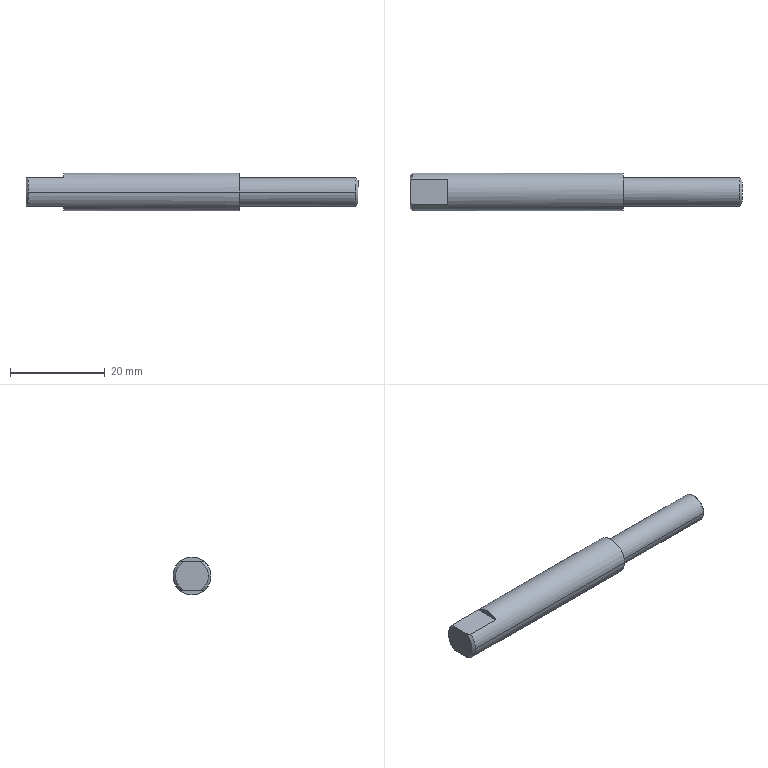Part | STEP file | 11-FG-B02611 | 1 solid | 15 faces | box 70 x 8 x 8 mm | volume 2907 mm3 | plane 7 | cylinder 4 | cone 4 | commonest cylinder face diameters 6 x2 8 x2
STEP:
#1=CARTESIAN_POINT('',(194.107,167.808,0.));
#2=VERTEX_POINT('',#1);
#3=CARTESIAN_POINT('',(194.107,175.808,0.));
#4=VERTEX_POINT('',#3);
#5=CARTESIAN_POINT('',(194.107,171.808,0.));
#6=DIRECTION('',(1.,0.,0.));
#7=DIRECTION('',(0.,0.,1.));
#8=AXIS2_PLACEMENT_3D('',#5,#6,#7);
#9=CIRCLE('',#8,4.);
#10=EDGE_CURVE('',#2,#4,#9,.T.);
#11=ORIENTED_EDGE('',*,*,#10,.F.);
#12=CARTESIAN_POINT('',(149.607,167.808,0.));
#13=VERTEX_POINT('',#12);
#14=CARTESIAN_POINT('',(194.107,167.808,0.));
#15=DIRECTION('',(-1.,0.,0.));
#16=VECTOR('',#15,1000.);
#17=LINE('',#14,#16);
#18=EDGE_CURVE('',#2,#13,#17,.T.);
#19=ORIENTED_EDGE('',*,*,#18,.T.);
#20=CARTESIAN_POINT('',(149.607,169.162,-3.));
#21=VERTEX_POINT('',#20);
#22=CARTESIAN_POINT('',(149.607,171.808,0.));
#23=DIRECTION('',(1.,0.,0.));
#24=DIRECTION('',(0.,0.,1.));
#25=AXIS2_PLACEMENT_3D('',#22,#23,#24);
#26=CIRCLE('',#25,4.);
#27=EDGE_CURVE('',#13,#21,#26,.T.);
#28=ORIENTED_EDGE('',*,*,#27,.T.);
#29=CARTESIAN_POINT('',(157.107,169.162,-3.));
#30=VERTEX_POINT('',#29);
#31=CARTESIAN_POINT('',(194.107,169.162,-3.));
#32=DIRECTION('',(1.,0.,0.));
#33=VECTOR('',#32,1000.);
#34=LINE('',#31,#33);
#35=EDGE_CURVE('',#21,#30,#34,.T.);
#36=ORIENTED_EDGE('',*,*,#35,.T.);
#37=CARTESIAN_POINT('',(157.107,174.454,-3.));
#38=VERTEX_POINT('',#37);
#39=CARTESIAN_POINT('',(157.107,171.808,0.));
#40=DIRECTION('',(1.,0.,0.));
#41=DIRECTION('',(0.,0.,1.));
#42=AXIS2_PLACEMENT_3D('',#39,#40,#41);
#43=CIRCLE('',#42,4.);
#44=EDGE_CURVE('',#30,#38,#43,.T.);
#45=ORIENTED_EDGE('',*,*,#44,.T.);
#46=CARTESIAN_POINT('',(149.607,174.454,-3.));
#47=VERTEX_POINT('',#46);
#48=CARTESIAN_POINT('',(194.107,174.454,-3.));
#49=DIRECTION('',(-1.,0.,0.));
#50=VECTOR('',#49,1000.);
#51=LINE('',#48,#50);
#52=EDGE_CURVE('',#38,#47,#51,.T.);
#53=ORIENTED_EDGE('',*,*,#52,.T.);
#54=CARTESIAN_POINT('',(149.607,175.808,0.));
#55=VERTEX_POINT('',#54);
#56=CARTESIAN_POINT('',(149.607,171.808,0.));
#57=DIRECTION('',(1.,0.,0.));
#58=DIRECTION('',(0.,0.,1.));
#59=AXIS2_PLACEMENT_3D('',#56,#57,#58);
#60=CIRCLE('',#59,4.);
#61=EDGE_CURVE('',#47,#55,#60,.T.);
#62=ORIENTED_EDGE('',*,*,#61,.T.);
#63=CARTESIAN_POINT('',(194.107,175.808,0.));
#64=DIRECTION('',(-1.,0.,0.));
#65=VECTOR('',#64,1000.);
#66=LINE('',#63,#65);
#67=EDGE_CURVE('',#4,#55,#66,.T.);
#68=ORIENTED_EDGE('',*,*,#67,.F.);
#69=EDGE_LOOP('',(#11,#19,#28,#36,#45,#53,#62,#68));
#70=FACE_OUTER_BOUND('',#69,.T.);
#71=CARTESIAN_POINT('',(194.107,171.808,0.));
#72=DIRECTION('',(-1.,0.,0.));
#73=DIRECTION('',(0.,1.,0.));
#74=AXIS2_PLACEMENT_3D('',#71,#72,#73);
#75=CYLINDRICAL_SURFACE('',#74,4.);
#76=ADVANCED_FACE('',(#70),#75,.T.);
#77=CARTESIAN_POINT('',(218.607,168.808,0.));
#78=VERTEX_POINT('',#77);
#79=CARTESIAN_POINT('',(218.607,171.808,-3.));
#80=VERTEX_POINT('',#79);
#81=CARTESIAN_POINT('',(218.607,171.808,0.));
#82=DIRECTION('',(1.,0.,0.));
#83=DIRECTION('',(0.,0.,1.));
#84=AXIS2_PLACEMENT_3D('',#81,#82,#83);
#85=CIRCLE('',#84,3.);
#86=EDGE_CURVE('',#78,#80,#85,.T.);
#87=ORIENTED_EDGE('',*,*,#86,.F.);
#88=CARTESIAN_POINT('',(194.107,168.808,0.));
#89=VERTEX_POINT('',#88);
#90=CARTESIAN_POINT('',(218.607,168.808,0.));
#91=DIRECTION('',(-1.,0.,0.));
#92=VECTOR('',#91,1000.);
#93=LINE('',#90,#92);
#94=EDGE_CURVE('',#78,#89,#93,.T.);
#95=ORIENTED_EDGE('',*,*,#94,.T.);
#96=CARTESIAN_POINT('',(194.107,174.808,0.));
#97=VERTEX_POINT('',#96);
#98=CARTESIAN_POINT('',(194.107,171.808,0.));
#99=DIRECTION('',(1.,0.,0.));
#100=DIRECTION('',(0.,0.,1.));
#101=AXIS2_PLACEMENT_3D('',#98,#99,#100);
#102=CIRCLE('',#101,3.);
#103=EDGE_CURVE('',#89,#97,#102,.T.);
#104=ORIENTED_EDGE('',*,*,#103,.T.);
#105=CARTESIAN_POINT('',(218.607,174.808,0.));
#106=VERTEX_POINT('',#105);
#107=CARTESIAN_POINT('',(218.607,174.808,0.));
#108=DIRECTION('',(-1.,0.,0.));
#109=VECTOR('',#108,1000.);
#110=LINE('',#107,#109);
#111=EDGE_CURVE('',#106,#97,#110,.T.);
#112=ORIENTED_EDGE('',*,*,#111,.F.);
#113=CARTESIAN_POINT('',(218.607,171.808,0.));
#114=DIRECTION('',(1.,0.,0.));
#115=DIRECTION('',(0.,0.,1.));
#116=AXIS2_PLACEMENT_3D('',#113,#114,#115);
#117=CIRCLE('',#116,3.);
#118=EDGE_CURVE('',#80,#106,#117,.T.);
#119=ORIENTED_EDGE('',*,*,#118,.F.);
#120=EDGE_LOOP('',(#87,#95,#104,#112,#119));
#121=FACE_OUTER_BOUND('',#120,.T.);
#122=CARTESIAN_POINT('',(218.607,171.808,0.));
#123=DIRECTION('',(-1.,0.,0.));
#124=DIRECTION('',(0.,1.,0.));
#125=AXIS2_PLACEMENT_3D('',#122,#123,#124);
#126=CYLINDRICAL_SURFACE('',#125,3.);
#127=ADVANCED_FACE('',(#121),#126,.T.);
#128=CARTESIAN_POINT('',(219.107,171.808,-2.5));
#129=VERTEX_POINT('',#128);
#130=CARTESIAN_POINT('',(219.107,171.808,2.5));
#131=VERTEX_POINT('',#130);
#132=CARTESIAN_POINT('',(219.107,171.808,0.));
#133=DIRECTION('',(1.,0.,0.));
#134=DIRECTION('',(0.,0.,1.));
#135=AXIS2_PLACEMENT_3D('',#132,#133,#134);
#136=CIRCLE('',#135,2.5);
#137=EDGE_CURVE('',#129,#131,#136,.T.);
#138=ORIENTED_EDGE('',*,*,#137,.F.);
#139=CARTESIAN_POINT('',(219.107,171.808,-2.5));
#140=DIRECTION('',(-0.7071,0.,-0.7071));
#141=VECTOR('',#140,1000.);
#142=LINE('',#139,#141);
#143=EDGE_CURVE('',#129,#80,#142,.T.);
#144=ORIENTED_EDGE('',*,*,#143,.T.);
#145=ORIENTED_EDGE('',*,*,#118,.T.);
#146=CARTESIAN_POINT('',(218.607,171.808,3.));
#147=VERTEX_POINT('',#146);
#148=CARTESIAN_POINT('',(218.607,171.808,0.));
#149=DIRECTION('',(1.,0.,0.));
#150=DIRECTION('',(0.,0.,1.));
#151=AXIS2_PLACEMENT_3D('',#148,#149,#150);
#152=CIRCLE('',#151,3.);
#153=EDGE_CURVE('',#106,#147,#152,.T.);
#154=ORIENTED_EDGE('',*,*,#153,.T.);
#155=CARTESIAN_POINT('',(219.107,171.808,2.5));
#156=DIRECTION('',(-0.7071,0.,0.7071));
#157=VECTOR('',#156,1000.);
#158=LINE('',#155,#157);
#159=EDGE_CURVE('',#131,#147,#158,.T.);
#160=ORIENTED_EDGE('',*,*,#159,.F.);
#161=EDGE_LOOP('',(#138,#144,#145,#154,#160));
#162=FACE_OUTER_BOUND('',#161,.T.);
#163=CARTESIAN_POINT('',(219.107,171.808,0.));
#164=DIRECTION('',(-1.,0.,0.));
#165=DIRECTION('',(0.,0.,1.));
#166=AXIS2_PLACEMENT_3D('',#163,#164,#165);
#167=CONICAL_SURFACE('',#166,2.5,0.7854);
#168=ADVANCED_FACE('',(#162),#167,.T.);
#169=CARTESIAN_POINT('',(219.107,171.808,0.));
#170=DIRECTION('',(1.,0.,0.));
#171=DIRECTION('',(0.,0.,1.));
#172=AXIS2_PLACEMENT_3D('',#169,#170,#171);
#173=CIRCLE('',#172,2.5);
#174=EDGE_CURVE('',#131,#129,#173,.T.);
#175=ORIENTED_EDGE('',*,*,#174,.T.);
#176=ORIENTED_EDGE('',*,*,#137,.T.);
#177=EDGE_LOOP('',(#175,#176));
#178=FACE_OUTER_BOUND('',#177,.T.);
#179=CARTESIAN_POINT('',(219.107,174.308,2.5));
#180=DIRECTION('',(1.,0.,0.));
#181=DIRECTION('',(0.,-1.,0.));
#182=AXIS2_PLACEMENT_3D('',#179,#180,#181);
#183=PLANE('',#182);
#184=ADVANCED_FACE('',(#178),#183,.T.);
#185=ORIENTED_EDGE('',*,*,#143,.F.);
#186=ORIENTED_EDGE('',*,*,#174,.F.);
#187=ORIENTED_EDGE('',*,*,#159,.T.);
#188=CARTESIAN_POINT('',(218.607,171.808,0.));
#189=DIRECTION('',(1.,0.,0.));
#190=DIRECTION('',(0.,0.,1.));
#191=AXIS2_PLACEMENT_3D('',#188,#189,#190);
#192=CIRCLE('',#191,3.);
#193=EDGE_CURVE('',#147,#78,#192,.T.);
#194=ORIENTED_EDGE('',*,*,#193,.T.);
#195=ORIENTED_EDGE('',*,*,#86,.T.);
#196=EDGE_LOOP('',(#185,#186,#187,#194,#195));
#197=FACE_OUTER_BOUND('',#196,.T.);
#198=CARTESIAN_POINT('',(219.107,171.808,0.));
#199=DIRECTION('',(-1.,0.,0.));
#200=DIRECTION('',(0.,0.,1.));
#201=AXIS2_PLACEMENT_3D('',#198,#199,#200);
#202=CONICAL_SURFACE('',#201,2.5,0.7854);
#203=ADVANCED_FACE('',(#197),#202,.T.);
#204=ORIENTED_EDGE('',*,*,#94,.F.);
#205=ORIENTED_EDGE('',*,*,#193,.F.);
#206=ORIENTED_EDGE('',*,*,#153,.F.);
#207=ORIENTED_EDGE('',*,*,#111,.T.);
#208=CARTESIAN_POINT('',(194.107,171.808,0.));
#209=DIRECTION('',(1.,0.,0.));
#210=DIRECTION('',(0.,0.,1.));
#211=AXIS2_PLACEMENT_3D('',#208,#209,#210);
#212=CIRCLE('',#211,3.);
#213=EDGE_CURVE('',#97,#89,#212,.T.);
#214=ORIENTED_EDGE('',*,*,#213,.T.);
#215=EDGE_LOOP('',(#204,#205,#206,#207,#214));
#216=FACE_OUTER_BOUND('',#215,.T.);
#217=CARTESIAN_POINT('',(218.607,171.808,0.));
#218=DIRECTION('',(-1.,0.,0.));
#219=DIRECTION('',(0.,1.,0.));
#220=AXIS2_PLACEMENT_3D('',#217,#218,#219);
#221=CYLINDRICAL_SURFACE('',#220,3.);
#222=ADVANCED_FACE('',(#216),#221,.T.);
#223=ORIENTED_EDGE('',*,*,#213,.F.);
#224=ORIENTED_EDGE('',*,*,#103,.F.);
#225=EDGE_LOOP('',(#223,#224));
#226=FACE_BOUND('',#225,.T.);
#227=CARTESIAN_POINT('',(194.107,171.808,0.));
#228=DIRECTION('',(1.,0.,0.));
#229=DIRECTION('',(0.,0.,1.));
#230=AXIS2_PLACEMENT_3D('',#227,#228,#229);
#231=CIRCLE('',#230,4.);
#232=EDGE_CURVE('',#4,#2,#231,.T.);
#233=ORIENTED_EDGE('',*,*,#232,.T.);
#234=ORIENTED_EDGE('',*,*,#10,.T.);
#235=EDGE_LOOP('',(#233,#234));
#236=FACE_OUTER_BOUND('',#235,.T.);
#237=CARTESIAN_POINT('',(194.107,175.808,4.));
#238=DIRECTION('',(1.,0.,0.));
#239=DIRECTION('',(0.,-1.,0.));
#240=AXIS2_PLACEMENT_3D('',#237,#238,#239);
#241=PLANE('',#240);
#242=ADVANCED_FACE('',(#226,#236),#241,.T.);
#243=ORIENTED_EDGE('',*,*,#18,.F.);
#244=ORIENTED_EDGE('',*,*,#232,.F.);
#245=ORIENTED_EDGE('',*,*,#67,.T.);
#246=CARTESIAN_POINT('',(149.607,174.454,3.));
#247=VERTEX_POINT('',#246);
#248=CARTESIAN_POINT('',(149.607,171.808,0.));
#249=DIRECTION('',(1.,0.,0.));
#250=DIRECTION('',(0.,0.,1.));
#251=AXIS2_PLACEMENT_3D('',#248,#249,#250);
#252=CIRCLE('',#251,4.);
#253=EDGE_CURVE('',#55,#247,#252,.T.);
#254=ORIENTED_EDGE('',*,*,#253,.T.);
#255=CARTESIAN_POINT('',(157.107,174.454,3.));
#256=VERTEX_POINT('',#255);
#257=CARTESIAN_POINT('',(194.107,174.454,3.));
#258=DIRECTION('',(1.,0.,0.));
#259=VECTOR('',#258,1000.);
#260=LINE('',#257,#259);
#261=EDGE_CURVE('',#247,#256,#260,.T.);
#262=ORIENTED_EDGE('',*,*,#261,.T.);
#263=CARTESIAN_POINT('',(157.107,169.162,3.));
#264=VERTEX_POINT('',#263);
#265=CARTESIAN_POINT('',(157.107,171.808,0.));
#266=DIRECTION('',(1.,0.,0.));
#267=DIRECTION('',(0.,0.,1.));
#268=AXIS2_PLACEMENT_3D('',#265,#266,#267);
#269=CIRCLE('',#268,4.);
#270=EDGE_CURVE('',#256,#264,#269,.T.);
#271=ORIENTED_EDGE('',*,*,#270,.T.);
#272=CARTESIAN_POINT('',(149.607,169.162,3.));
#273=VERTEX_POINT('',#272);
#274=CARTESIAN_POINT('',(194.107,169.162,3.));
#275=DIRECTION('',(-1.,0.,0.));
#276=VECTOR('',#275,1000.);
#277=LINE('',#274,#276);
#278=EDGE_CURVE('',#264,#273,#277,.T.);
#279=ORIENTED_EDGE('',*,*,#278,.T.);
#280=CARTESIAN_POINT('',(149.607,171.808,0.));
#281=DIRECTION('',(1.,0.,0.));
#282=DIRECTION('',(0.,0.,1.));
#283=AXIS2_PLACEMENT_3D('',#280,#281,#282);
#284=CIRCLE('',#283,4.);
#285=EDGE_CURVE('',#273,#13,#284,.T.);
#286=ORIENTED_EDGE('',*,*,#285,.T.);
#287=EDGE_LOOP('',(#243,#244,#245,#254,#262,#271,#279,#286));
#288=FACE_OUTER_BOUND('',#287,.T.);
#289=CARTESIAN_POINT('',(194.107,171.808,0.));
#290=DIRECTION('',(-1.,0.,0.));
#291=DIRECTION('',(0.,1.,0.));
#292=AXIS2_PLACEMENT_3D('',#289,#290,#291);
#293=CYLINDRICAL_SURFACE('',#292,4.);
#294=ADVANCED_FACE('',(#288),#293,.T.);
#295=CARTESIAN_POINT('',(149.107,170.005,-3.));
#296=VERTEX_POINT('',#295);
#297=CARTESIAN_POINT('',(149.107,170.005,-3.));
#298=CARTESIAN_POINT('',(149.257,169.714,-3.));
#299=CARTESIAN_POINT('',(149.426,169.435,-3.));
#300=CARTESIAN_POINT('',(149.607,169.162,-3.));
#301=B_SPLINE_CURVE_WITH_KNOTS('',3,(#297,#298,#299,#300),.UNSPECIFIED.,.F.,.F.,(4,4),(0.,0.0009801),.UNSPECIFIED.);
#302=EDGE_CURVE('',#296,#21,#301,.T.);
#303=ORIENTED_EDGE('',*,*,#302,.F.);
#304=CARTESIAN_POINT('',(149.107,173.611,-3.));
#305=VERTEX_POINT('',#304);
#306=CARTESIAN_POINT('',(149.107,167.805,-3.));
#307=DIRECTION('',(0.,-1.,0.));
#308=VECTOR('',#307,1000.);
#309=LINE('',#306,#308);
#310=EDGE_CURVE('',#305,#296,#309,.T.);
#311=ORIENTED_EDGE('',*,*,#310,.F.);
#312=CARTESIAN_POINT('',(149.607,174.454,-3.));
#313=CARTESIAN_POINT('',(149.426,174.181,-3.));
#314=CARTESIAN_POINT('',(149.257,173.902,-3.));
#315=CARTESIAN_POINT('',(149.107,173.611,-3.));
#316=B_SPLINE_CURVE_WITH_KNOTS('',3,(#312,#313,#314,#315),.UNSPECIFIED.,.F.,.F.,(4,4),(0.,0.0009801),.UNSPECIFIED.);
#317=EDGE_CURVE('',#47,#305,#316,.T.);
#318=ORIENTED_EDGE('',*,*,#317,.F.);
#319=ORIENTED_EDGE('',*,*,#52,.F.);
#320=CARTESIAN_POINT('',(157.107,174.954,-3.));
#321=DIRECTION('',(0.,1.,0.));
#322=VECTOR('',#321,1000.);
#323=LINE('',#320,#322);
#324=EDGE_CURVE('',#30,#38,#323,.T.);
#325=ORIENTED_EDGE('',*,*,#324,.F.);
#326=ORIENTED_EDGE('',*,*,#35,.F.);
#327=EDGE_LOOP('',(#303,#311,#318,#319,#325,#326));
#328=FACE_OUTER_BOUND('',#327,.T.);
#329=CARTESIAN_POINT('',(149.101,174.458,-3.));
#330=DIRECTION('',(0.,0.,1.));
#331=DIRECTION('',(0.,-1.,0.));
#332=AXIS2_PLACEMENT_3D('',#329,#330,#331);
#333=PLANE('',#332);
#334=ADVANCED_FACE('',(#328),#333,.F.);
#335=ORIENTED_EDGE('',*,*,#44,.F.);
#336=ORIENTED_EDGE('',*,*,#324,.T.);
#337=EDGE_LOOP('',(#335,#336));
#338=FACE_OUTER_BOUND('',#337,.T.);
#339=CARTESIAN_POINT('',(157.107,174.954,-4.502));
#340=DIRECTION('',(-1.,0.,0.));
#341=DIRECTION('',(0.,-1.,0.));
#342=AXIS2_PLACEMENT_3D('',#339,#340,#341);
#343=PLANE('',#342);
#344=ADVANCED_FACE('',(#338),#343,.T.);
#345=CARTESIAN_POINT('',(149.107,170.005,3.));
#346=VERTEX_POINT('',#345);
#347=CARTESIAN_POINT('',(149.607,169.162,3.));
#348=CARTESIAN_POINT('',(149.426,169.435,3.));
#349=CARTESIAN_POINT('',(149.257,169.714,3.));
#350=CARTESIAN_POINT('',(149.107,170.005,3.));
#351=B_SPLINE_CURVE_WITH_KNOTS('',3,(#347,#348,#349,#350),.UNSPECIFIED.,.F.,.F.,(4,4),(0.,0.0009801),.UNSPECIFIED.);
#352=EDGE_CURVE('',#273,#346,#351,.T.);
#353=ORIENTED_EDGE('',*,*,#352,.T.);
#354=CARTESIAN_POINT('',(149.107,171.808,0.));
#355=DIRECTION('',(1.,0.,0.));
#356=DIRECTION('',(0.,0.,-1.));
#357=AXIS2_PLACEMENT_3D('',#354,#355,#356);
#358=CIRCLE('',#357,3.5);
#359=EDGE_CURVE('',#346,#296,#358,.T.);
#360=ORIENTED_EDGE('',*,*,#359,.T.);
#361=ORIENTED_EDGE('',*,*,#302,.T.);
#362=ORIENTED_EDGE('',*,*,#27,.F.);
#363=ORIENTED_EDGE('',*,*,#285,.F.);
#364=EDGE_LOOP('',(#353,#360,#361,#362,#363));
#365=FACE_OUTER_BOUND('',#364,.T.);
#366=CARTESIAN_POINT('',(149.615,171.808,0.));
#367=DIRECTION('',(1.,0.,0.));
#368=DIRECTION('',(0.,0.,-1.));
#369=AXIS2_PLACEMENT_3D('',#366,#367,#368);
#370=CONICAL_SURFACE('',#369,4.008,0.7854);
#371=ADVANCED_FACE('',(#365),#370,.T.);
#372=CARTESIAN_POINT('',(149.107,173.611,3.));
#373=VERTEX_POINT('',#372);
#374=CARTESIAN_POINT('',(149.107,173.611,3.));
#375=CARTESIAN_POINT('',(149.257,173.902,3.));
#376=CARTESIAN_POINT('',(149.426,174.181,3.));
#377=CARTESIAN_POINT('',(149.607,174.454,3.));
#378=B_SPLINE_CURVE_WITH_KNOTS('',3,(#374,#375,#376,#377),.UNSPECIFIED.,.F.,.F.,(4,4),(0.,0.0009801),.UNSPECIFIED.);
#379=EDGE_CURVE('',#373,#247,#378,.T.);
#380=ORIENTED_EDGE('',*,*,#379,.F.);
#381=CARTESIAN_POINT('',(149.107,167.805,3.));
#382=DIRECTION('',(0.,1.,0.));
#383=VECTOR('',#382,1000.);
#384=LINE('',#381,#383);
#385=EDGE_CURVE('',#346,#373,#384,.T.);
#386=ORIENTED_EDGE('',*,*,#385,.F.);
#387=ORIENTED_EDGE('',*,*,#352,.F.);
#388=ORIENTED_EDGE('',*,*,#278,.F.);
#389=CARTESIAN_POINT('',(157.107,174.954,3.));
#390=DIRECTION('',(0.,-1.,0.));
#391=VECTOR('',#390,1000.);
#392=LINE('',#389,#391);
#393=EDGE_CURVE('',#256,#264,#392,.T.);
#394=ORIENTED_EDGE('',*,*,#393,.F.);
#395=ORIENTED_EDGE('',*,*,#261,.F.);
#396=EDGE_LOOP('',(#380,#386,#387,#388,#394,#395));
#397=FACE_OUTER_BOUND('',#396,.T.);
#398=CARTESIAN_POINT('',(149.101,169.158,3.));
#399=DIRECTION('',(0.,0.,-1.));
#400=DIRECTION('',(0.,1.,0.));
#401=AXIS2_PLACEMENT_3D('',#398,#399,#400);
#402=PLANE('',#401);
#403=ADVANCED_FACE('',(#397),#402,.F.);
#404=ORIENTED_EDGE('',*,*,#270,.F.);
#405=ORIENTED_EDGE('',*,*,#393,.T.);
#406=EDGE_LOOP('',(#404,#405));
#407=FACE_OUTER_BOUND('',#406,.T.);
#408=CARTESIAN_POINT('',(157.107,174.954,2.767));
#409=DIRECTION('',(-1.,0.,0.));
#410=DIRECTION('',(0.,-1.,0.));
#411=AXIS2_PLACEMENT_3D('',#408,#409,#410);
#412=PLANE('',#411);
#413=ADVANCED_FACE('',(#407),#412,.T.);
#414=ORIENTED_EDGE('',*,*,#61,.F.);
#415=ORIENTED_EDGE('',*,*,#317,.T.);
#416=CARTESIAN_POINT('',(149.107,171.808,0.));
#417=DIRECTION('',(1.,0.,0.));
#418=DIRECTION('',(0.,0.,-1.));
#419=AXIS2_PLACEMENT_3D('',#416,#417,#418);
#420=CIRCLE('',#419,3.5);
#421=EDGE_CURVE('',#305,#373,#420,.T.);
#422=ORIENTED_EDGE('',*,*,#421,.T.);
#423=ORIENTED_EDGE('',*,*,#379,.T.);
#424=ORIENTED_EDGE('',*,*,#253,.F.);
#425=EDGE_LOOP('',(#414,#415,#422,#423,#424));
#426=FACE_OUTER_BOUND('',#425,.T.);
#427=CARTESIAN_POINT('',(149.615,171.808,0.));
#428=DIRECTION('',(1.,0.,0.));
#429=DIRECTION('',(0.,0.,-1.));
#430=AXIS2_PLACEMENT_3D('',#427,#428,#429);
#431=CONICAL_SURFACE('',#430,4.008,0.7854);
#432=ADVANCED_FACE('',(#426),#431,.T.);
#433=ORIENTED_EDGE('',*,*,#359,.F.);
#434=ORIENTED_EDGE('',*,*,#385,.T.);
#435=ORIENTED_EDGE('',*,*,#421,.F.);
#436=ORIENTED_EDGE('',*,*,#310,.T.);
#437=EDGE_LOOP('',(#433,#434,#435,#436));
#438=FACE_OUTER_BOUND('',#437,.T.);
#439=CARTESIAN_POINT('',(149.107,167.805,3.5));
#440=DIRECTION('',(-1.,0.,0.));
#441=DIRECTION('',(0.,1.,0.));
#442=AXIS2_PLACEMENT_3D('',#439,#440,#441);
#443=PLANE('',#442);
#444=ADVANCED_FACE('',(#438),#443,.T.);
#445=CLOSED_SHELL('',(#76,#127,#168,#184,#203,#222,#242,#294,#334,#344,#371,#403,#413,#432,#444));
#446=MANIFOLD_SOLID_BREP('',#445);
#447=CARTESIAN_POINT('',(0.,0.,0.));
#448=DIRECTION('',(0.,0.,1.));
#449=DIRECTION('',(1.,0.,0.));
#450=AXIS2_PLACEMENT_3D('',#447,#448,#449);
#451=(LENGTH_UNIT()NAMED_UNIT(*)SI_UNIT(.MILLI.,.METRE.));
#452=UNCERTAINTY_MEASURE_WITH_UNIT(LENGTH_MEASURE(0.00001),#451,'','');
#453=(NAMED_UNIT(*)PLANE_ANGLE_UNIT()SI_UNIT($,.RADIAN.));
#454=(NAMED_UNIT(*)SI_UNIT($,.STERADIAN.)SOLID_ANGLE_UNIT());
#455=(GEOMETRIC_REPRESENTATION_CONTEXT(3)GLOBAL_UNCERTAINTY_ASSIGNED_CONTEXT((#452))GLOBAL_UNIT_ASSIGNED_CONTEXT((#451,#453,#454))REPRESENTATION_CONTEXT('',''));
#456=ADVANCED_BREP_SHAPE_REPRESENTATION('',(#446,#450),#455);